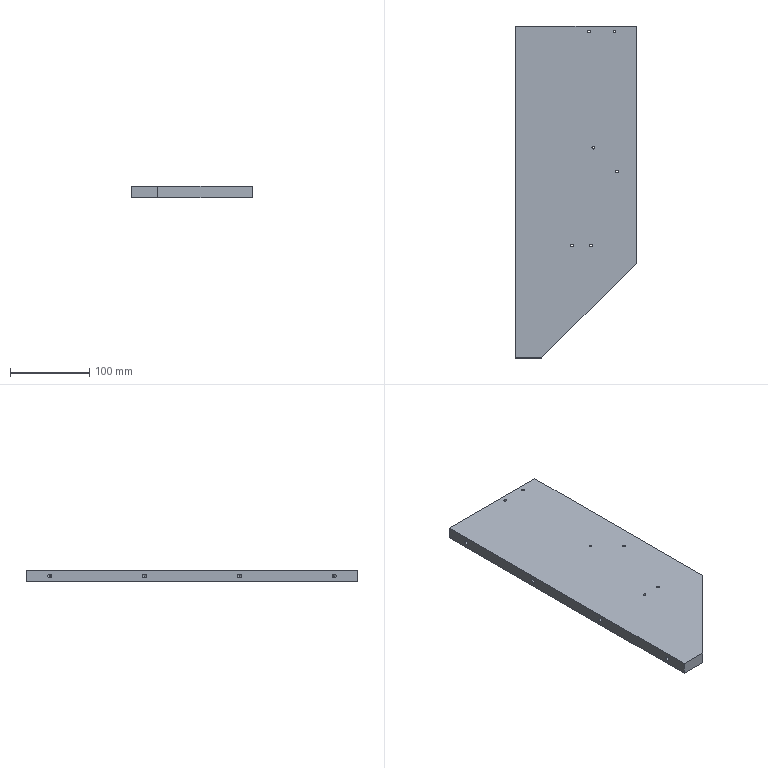Part | STEP file | KF-2212-050-006 | 1 solid | 51 faces | box 153 x 420 x 15 mm | volume 852381 mm3 | cylinder 28 | cone 16 | plane 7 | commonest cylinder face diameters 5 x16 3.3 x12
STEP:
#1=CARTESIAN_POINT('',(-3.35,-67.65,15.));
#2=VERTEX_POINT('',#1);
#3=CARTESIAN_POINT('',(-6.65,-67.65,15.));
#4=VERTEX_POINT('',#3);
#5=CARTESIAN_POINT('',(-5.,-67.65,15.));
#6=DIRECTION('',(0.,0.,-1.));
#7=DIRECTION('',(-1.,0.,0.));
#8=AXIS2_PLACEMENT_3D('',#5,#6,#7);
#9=CIRCLE('',#8,1.65);
#10=EDGE_CURVE('',#2,#4,#9,.T.);
#11=ORIENTED_EDGE('',*,*,#10,.F.);
#12=CARTESIAN_POINT('',(-3.35,-67.65,0.));
#13=VERTEX_POINT('',#12);
#14=CARTESIAN_POINT('',(-3.35,-67.65,0.));
#15=DIRECTION('',(0.,0.,-1.));
#16=VECTOR('',#15,1000.);
#17=LINE('',#14,#16);
#18=EDGE_CURVE('',#2,#13,#17,.T.);
#19=ORIENTED_EDGE('',*,*,#18,.T.);
#20=CARTESIAN_POINT('',(-6.65,-67.65,0.));
#21=VERTEX_POINT('',#20);
#22=CARTESIAN_POINT('',(-5.,-67.65,0.));
#23=DIRECTION('',(0.,0.,-1.));
#24=DIRECTION('',(-1.,0.,0.));
#25=AXIS2_PLACEMENT_3D('',#22,#23,#24);
#26=CIRCLE('',#25,1.65);
#27=EDGE_CURVE('',#13,#21,#26,.T.);
#28=ORIENTED_EDGE('',*,*,#27,.T.);
#29=CARTESIAN_POINT('',(-6.65,-67.65,0.));
#30=DIRECTION('',(0.,0.,-1.));
#31=VECTOR('',#30,1000.);
#32=LINE('',#29,#31);
#33=EDGE_CURVE('',#4,#21,#32,.T.);
#34=ORIENTED_EDGE('',*,*,#33,.F.);
#35=EDGE_LOOP('',(#11,#19,#28,#34));
#36=FACE_OUTER_BOUND('',#35,.T.);
#37=CARTESIAN_POINT('',(-5.,-67.65,0.));
#38=DIRECTION('',(0.,0.,-1.));
#39=DIRECTION('',(-1.,0.,0.));
#40=AXIS2_PLACEMENT_3D('',#37,#38,#39);
#41=CYLINDRICAL_SURFACE('',#40,1.65);
#42=ADVANCED_FACE('',(#36),#41,.F.);
#43=CARTESIAN_POINT('',(20.65,-67.65,15.));
#44=VERTEX_POINT('',#43);
#45=CARTESIAN_POINT('',(17.35,-67.65,15.));
#46=VERTEX_POINT('',#45);
#47=CARTESIAN_POINT('',(19.,-67.65,15.));
#48=DIRECTION('',(0.,0.,-1.));
#49=DIRECTION('',(-1.,0.,0.));
#50=AXIS2_PLACEMENT_3D('',#47,#48,#49);
#51=CIRCLE('',#50,1.65);
#52=EDGE_CURVE('',#44,#46,#51,.T.);
#53=ORIENTED_EDGE('',*,*,#52,.F.);
#54=CARTESIAN_POINT('',(20.65,-67.65,0.));
#55=VERTEX_POINT('',#54);
#56=CARTESIAN_POINT('',(20.65,-67.65,0.));
#57=DIRECTION('',(0.,0.,-1.));
#58=VECTOR('',#57,1000.);
#59=LINE('',#56,#58);
#60=EDGE_CURVE('',#44,#55,#59,.T.);
#61=ORIENTED_EDGE('',*,*,#60,.T.);
#62=CARTESIAN_POINT('',(17.35,-67.65,0.));
#63=VERTEX_POINT('',#62);
#64=CARTESIAN_POINT('',(19.,-67.65,0.));
#65=DIRECTION('',(0.,0.,-1.));
#66=DIRECTION('',(-1.,0.,0.));
#67=AXIS2_PLACEMENT_3D('',#64,#65,#66);
#68=CIRCLE('',#67,1.65);
#69=EDGE_CURVE('',#55,#63,#68,.T.);
#70=ORIENTED_EDGE('',*,*,#69,.T.);
#71=CARTESIAN_POINT('',(17.35,-67.65,0.));
#72=DIRECTION('',(0.,0.,-1.));
#73=VECTOR('',#72,1000.);
#74=LINE('',#71,#73);
#75=EDGE_CURVE('',#46,#63,#74,.T.);
#76=ORIENTED_EDGE('',*,*,#75,.F.);
#77=EDGE_LOOP('',(#53,#61,#70,#76));
#78=FACE_OUTER_BOUND('',#77,.T.);
#79=CARTESIAN_POINT('',(19.,-67.65,0.));
#80=DIRECTION('',(0.,0.,-1.));
#81=DIRECTION('',(-1.,0.,0.));
#82=AXIS2_PLACEMENT_3D('',#79,#80,#81);
#83=CYLINDRICAL_SURFACE('',#82,1.65);
#84=ADVANCED_FACE('',(#78),#83,.F.);
#85=CARTESIAN_POINT('',(23.523,56.,15.));
#86=VERTEX_POINT('',#85);
#87=CARTESIAN_POINT('',(20.223,56.,15.));
#88=VERTEX_POINT('',#87);
#89=CARTESIAN_POINT('',(21.873,56.,15.));
#90=DIRECTION('',(0.,0.,-1.));
#91=DIRECTION('',(-1.,0.,0.));
#92=AXIS2_PLACEMENT_3D('',#89,#90,#91);
#93=CIRCLE('',#92,1.65);
#94=EDGE_CURVE('',#86,#88,#93,.T.);
#95=ORIENTED_EDGE('',*,*,#94,.F.);
#96=CARTESIAN_POINT('',(23.523,56.,0.));
#97=VERTEX_POINT('',#96);
#98=CARTESIAN_POINT('',(23.523,56.,0.));
#99=DIRECTION('',(0.,0.,-1.));
#100=VECTOR('',#99,1000.);
#101=LINE('',#98,#100);
#102=EDGE_CURVE('',#86,#97,#101,.T.);
#103=ORIENTED_EDGE('',*,*,#102,.T.);
#104=CARTESIAN_POINT('',(20.223,56.,0.));
#105=VERTEX_POINT('',#104);
#106=CARTESIAN_POINT('',(21.873,56.,0.));
#107=DIRECTION('',(0.,0.,-1.));
#108=DIRECTION('',(-1.,0.,0.));
#109=AXIS2_PLACEMENT_3D('',#106,#107,#108);
#110=CIRCLE('',#109,1.65);
#111=EDGE_CURVE('',#97,#105,#110,.T.);
#112=ORIENTED_EDGE('',*,*,#111,.T.);
#113=CARTESIAN_POINT('',(20.223,56.,0.));
#114=DIRECTION('',(0.,0.,-1.));
#115=VECTOR('',#114,1000.);
#116=LINE('',#113,#115);
#117=EDGE_CURVE('',#88,#105,#116,.T.);
#118=ORIENTED_EDGE('',*,*,#117,.F.);
#119=EDGE_LOOP('',(#95,#103,#112,#118));
#120=FACE_OUTER_BOUND('',#119,.T.);
#121=CARTESIAN_POINT('',(21.873,56.,0.));
#122=DIRECTION('',(0.,0.,-1.));
#123=DIRECTION('',(-1.,0.,0.));
#124=AXIS2_PLACEMENT_3D('',#121,#122,#123);
#125=CYLINDRICAL_SURFACE('',#124,1.65);
#126=ADVANCED_FACE('',(#120),#125,.F.);
#127=CARTESIAN_POINT('',(53.523,26.,15.));
#128=VERTEX_POINT('',#127);
#129=CARTESIAN_POINT('',(50.223,26.,15.));
#130=VERTEX_POINT('',#129);
#131=CARTESIAN_POINT('',(51.873,26.,15.));
#132=DIRECTION('',(0.,0.,-1.));
#133=DIRECTION('',(-1.,0.,0.));
#134=AXIS2_PLACEMENT_3D('',#131,#132,#133);
#135=CIRCLE('',#134,1.65);
#136=EDGE_CURVE('',#128,#130,#135,.T.);
#137=ORIENTED_EDGE('',*,*,#136,.F.);
#138=CARTESIAN_POINT('',(53.523,26.,0.));
#139=VERTEX_POINT('',#138);
#140=CARTESIAN_POINT('',(53.523,26.,0.));
#141=DIRECTION('',(0.,0.,-1.));
#142=VECTOR('',#141,1000.);
#143=LINE('',#140,#142);
#144=EDGE_CURVE('',#128,#139,#143,.T.);
#145=ORIENTED_EDGE('',*,*,#144,.T.);
#146=CARTESIAN_POINT('',(50.223,26.,0.));
#147=VERTEX_POINT('',#146);
#148=CARTESIAN_POINT('',(51.873,26.,0.));
#149=DIRECTION('',(0.,0.,-1.));
#150=DIRECTION('',(-1.,0.,0.));
#151=AXIS2_PLACEMENT_3D('',#148,#149,#150);
#152=CIRCLE('',#151,1.65);
#153=EDGE_CURVE('',#139,#147,#152,.T.);
#154=ORIENTED_EDGE('',*,*,#153,.T.);
#155=CARTESIAN_POINT('',(50.223,26.,0.));
#156=DIRECTION('',(0.,0.,-1.));
#157=VECTOR('',#156,1000.);
#158=LINE('',#155,#157);
#159=EDGE_CURVE('',#130,#147,#158,.T.);
#160=ORIENTED_EDGE('',*,*,#159,.F.);
#161=EDGE_LOOP('',(#137,#145,#154,#160));
#162=FACE_OUTER_BOUND('',#161,.T.);
#163=CARTESIAN_POINT('',(51.873,26.,0.));
#164=DIRECTION('',(0.,0.,-1.));
#165=DIRECTION('',(-1.,0.,0.));
#166=AXIS2_PLACEMENT_3D('',#163,#164,#165);
#167=CYLINDRICAL_SURFACE('',#166,1.65);
#168=ADVANCED_FACE('',(#162),#167,.F.);
#169=CARTESIAN_POINT('',(18.15,203.,15.));
#170=VERTEX_POINT('',#169);
#171=CARTESIAN_POINT('',(14.85,203.,15.));
#172=VERTEX_POINT('',#171);
#173=CARTESIAN_POINT('',(16.5,203.,15.));
#174=DIRECTION('',(0.,0.,-1.));
#175=DIRECTION('',(-1.,0.,0.));
#176=AXIS2_PLACEMENT_3D('',#173,#174,#175);
#177=CIRCLE('',#176,1.65);
#178=EDGE_CURVE('',#170,#172,#177,.T.);
#179=ORIENTED_EDGE('',*,*,#178,.F.);
#180=CARTESIAN_POINT('',(18.15,203.,0.));
#181=VERTEX_POINT('',#180);
#182=CARTESIAN_POINT('',(18.15,203.,0.));
#183=DIRECTION('',(0.,0.,-1.));
#184=VECTOR('',#183,1000.);
#185=LINE('',#182,#184);
#186=EDGE_CURVE('',#170,#181,#185,.T.);
#187=ORIENTED_EDGE('',*,*,#186,.T.);
#188=CARTESIAN_POINT('',(14.85,203.,0.));
#189=VERTEX_POINT('',#188);
#190=CARTESIAN_POINT('',(16.5,203.,0.));
#191=DIRECTION('',(0.,0.,-1.));
#192=DIRECTION('',(-1.,0.,0.));
#193=AXIS2_PLACEMENT_3D('',#190,#191,#192);
#194=CIRCLE('',#193,1.65);
#195=EDGE_CURVE('',#181,#189,#194,.T.);
#196=ORIENTED_EDGE('',*,*,#195,.T.);
#197=CARTESIAN_POINT('',(14.85,203.,0.));
#198=DIRECTION('',(0.,0.,-1.));
#199=VECTOR('',#198,1000.);
#200=LINE('',#197,#199);
#201=EDGE_CURVE('',#172,#189,#200,.T.);
#202=ORIENTED_EDGE('',*,*,#201,.F.);
#203=EDGE_LOOP('',(#179,#187,#196,#202));
#204=FACE_OUTER_BOUND('',#203,.T.);
#205=CARTESIAN_POINT('',(16.5,203.,0.));
#206=DIRECTION('',(0.,0.,-1.));
#207=DIRECTION('',(-1.,0.,0.));
#208=AXIS2_PLACEMENT_3D('',#205,#206,#207);
#209=CYLINDRICAL_SURFACE('',#208,1.65);
#210=ADVANCED_FACE('',(#204),#209,.F.);
#211=CARTESIAN_POINT('',(50.15,203.,15.));
#212=VERTEX_POINT('',#211);
#213=CARTESIAN_POINT('',(46.85,203.,15.));
#214=VERTEX_POINT('',#213);
#215=CARTESIAN_POINT('',(48.5,203.,15.));
#216=DIRECTION('',(0.,0.,-1.));
#217=DIRECTION('',(-1.,0.,0.));
#218=AXIS2_PLACEMENT_3D('',#215,#216,#217);
#219=CIRCLE('',#218,1.65);
#220=EDGE_CURVE('',#212,#214,#219,.T.);
#221=ORIENTED_EDGE('',*,*,#220,.F.);
#222=CARTESIAN_POINT('',(50.15,203.,0.));
#223=VERTEX_POINT('',#222);
#224=CARTESIAN_POINT('',(50.15,203.,0.));
#225=DIRECTION('',(0.,0.,-1.));
#226=VECTOR('',#225,1000.);
#227=LINE('',#224,#226);
#228=EDGE_CURVE('',#212,#223,#227,.T.);
#229=ORIENTED_EDGE('',*,*,#228,.T.);
#230=CARTESIAN_POINT('',(46.85,203.,0.));
#231=VERTEX_POINT('',#230);
#232=CARTESIAN_POINT('',(48.5,203.,0.));
#233=DIRECTION('',(0.,0.,-1.));
#234=DIRECTION('',(-1.,0.,0.));
#235=AXIS2_PLACEMENT_3D('',#232,#233,#234);
#236=CIRCLE('',#235,1.65);
#237=EDGE_CURVE('',#223,#231,#236,.T.);
#238=ORIENTED_EDGE('',*,*,#237,.T.);
#239=CARTESIAN_POINT('',(46.85,203.,0.));
#240=DIRECTION('',(0.,0.,-1.));
#241=VECTOR('',#240,1000.);
#242=LINE('',#239,#241);
#243=EDGE_CURVE('',#214,#231,#242,.T.);
#244=ORIENTED_EDGE('',*,*,#243,.F.);
#245=EDGE_LOOP('',(#221,#229,#238,#244));
#246=FACE_OUTER_BOUND('',#245,.T.);
#247=CARTESIAN_POINT('',(48.5,203.,0.));
#248=DIRECTION('',(0.,0.,-1.));
#249=DIRECTION('',(-1.,0.,0.));
#250=AXIS2_PLACEMENT_3D('',#247,#248,#249);
#251=CYLINDRICAL_SURFACE('',#250,1.65);
#252=ADVANCED_FACE('',(#246),#251,.F.);
#253=CARTESIAN_POINT('',(59.5,-75.,10.));
#254=VERTEX_POINT('',#253);
#255=CARTESIAN_POINT('',(59.5,-75.,5.));
#256=VERTEX_POINT('',#255);
#257=CARTESIAN_POINT('',(59.5,-75.,7.5));
#258=DIRECTION('',(1.,0.,0.));
#259=DIRECTION('',(0.,0.,-1.));
#260=AXIS2_PLACEMENT_3D('',#257,#258,#259);
#261=CIRCLE('',#260,2.5);
#262=EDGE_CURVE('',#254,#256,#261,.T.);
#263=ORIENTED_EDGE('',*,*,#262,.F.);
#264=CARTESIAN_POINT('',(76.5,-75.,10.));
#265=VERTEX_POINT('',#264);
#266=CARTESIAN_POINT('',(76.5,-75.,10.));
#267=DIRECTION('',(1.,0.,0.));
#268=VECTOR('',#267,1000.);
#269=LINE('',#266,#268);
#270=EDGE_CURVE('',#254,#265,#269,.T.);
#271=ORIENTED_EDGE('',*,*,#270,.T.);
#272=CARTESIAN_POINT('',(76.5,-75.,5.));
#273=VERTEX_POINT('',#272);
#274=CARTESIAN_POINT('',(76.5,-75.,7.5));
#275=DIRECTION('',(1.,0.,0.));
#276=DIRECTION('',(0.,0.,-1.));
#277=AXIS2_PLACEMENT_3D('',#274,#275,#276);
#278=CIRCLE('',#277,2.5);
#279=EDGE_CURVE('',#265,#273,#278,.T.);
#280=ORIENTED_EDGE('',*,*,#279,.T.);
#281=CARTESIAN_POINT('',(76.5,-75.,5.));
#282=DIRECTION('',(1.,0.,0.));
#283=VECTOR('',#282,1000.);
#284=LINE('',#281,#283);
#285=EDGE_CURVE('',#256,#273,#284,.T.);
#286=ORIENTED_EDGE('',*,*,#285,.F.);
#287=EDGE_LOOP('',(#263,#271,#280,#286));
#288=FACE_OUTER_BOUND('',#287,.T.);
#289=CARTESIAN_POINT('',(76.5,-75.,7.5));
#290=DIRECTION('',(1.,0.,0.));
#291=DIRECTION('',(0.,0.,-1.));
#292=AXIS2_PLACEMENT_3D('',#289,#290,#291);
#293=CYLINDRICAL_SURFACE('',#292,2.5);
#294=ADVANCED_FACE('',(#288),#293,.F.);
#295=CARTESIAN_POINT('',(57.998,-75.,7.5));
#296=VERTEX_POINT('',#295);
#297=CARTESIAN_POINT('',(59.5,-75.,5.));
#298=DIRECTION('',(0.515,0.,-0.8572));
#299=VECTOR('',#298,1000.);
#300=LINE('',#297,#299);
#301=EDGE_CURVE('',#296,#256,#300,.T.);
#302=ORIENTED_EDGE('',*,*,#301,.F.);
#303=CARTESIAN_POINT('',(59.5,-75.,10.));
#304=DIRECTION('',(0.515,0.,0.8572));
#305=VECTOR('',#304,1000.);
#306=LINE('',#303,#305);
#307=EDGE_CURVE('',#296,#254,#306,.T.);
#308=ORIENTED_EDGE('',*,*,#307,.T.);
#309=ORIENTED_EDGE('',*,*,#262,.T.);
#310=EDGE_LOOP('',(#302,#308,#309));
#311=FACE_OUTER_BOUND('',#310,.T.);
#312=CARTESIAN_POINT('',(59.5,-75.,7.5));
#313=DIRECTION('',(1.,0.,0.));
#314=DIRECTION('',(0.,0.,-1.));
#315=AXIS2_PLACEMENT_3D('',#312,#313,#314);
#316=CONICAL_SURFACE('',#315,2.5,1.03);
#317=ADVANCED_FACE('',(#311),#316,.F.);
#318=CARTESIAN_POINT('',(59.5,15.,10.));
#319=VERTEX_POINT('',#318);
#320=CARTESIAN_POINT('',(59.5,15.,5.));
#321=VERTEX_POINT('',#320);
#322=CARTESIAN_POINT('',(59.5,15.,7.5));
#323=DIRECTION('',(1.,0.,0.));
#324=DIRECTION('',(0.,0.,-1.));
#325=AXIS2_PLACEMENT_3D('',#322,#323,#324);
#326=CIRCLE('',#325,2.5);
#327=EDGE_CURVE('',#319,#321,#326,.T.);
#328=ORIENTED_EDGE('',*,*,#327,.F.);
#329=CARTESIAN_POINT('',(76.5,15.,10.));
#330=VERTEX_POINT('',#329);
#331=CARTESIAN_POINT('',(76.5,15.,10.));
#332=DIRECTION('',(1.,0.,0.));
#333=VECTOR('',#332,1000.);
#334=LINE('',#331,#333);
#335=EDGE_CURVE('',#319,#330,#334,.T.);
#336=ORIENTED_EDGE('',*,*,#335,.T.);
#337=CARTESIAN_POINT('',(76.5,15.,5.));
#338=VERTEX_POINT('',#337);
#339=CARTESIAN_POINT('',(76.5,15.,7.5));
#340=DIRECTION('',(1.,0.,0.));
#341=DIRECTION('',(0.,0.,-1.));
#342=AXIS2_PLACEMENT_3D('',#339,#340,#341);
#343=CIRCLE('',#342,2.5);
#344=EDGE_CURVE('',#330,#338,#343,.T.);
#345=ORIENTED_EDGE('',*,*,#344,.T.);
#346=CARTESIAN_POINT('',(76.5,15.,5.));
#347=DIRECTION('',(1.,0.,0.));
#348=VECTOR('',#347,1000.);
#349=LINE('',#346,#348);
#350=EDGE_CURVE('',#321,#338,#349,.T.);
#351=ORIENTED_EDGE('',*,*,#350,.F.);
#352=EDGE_LOOP('',(#328,#336,#345,#351));
#353=FACE_OUTER_BOUND('',#352,.T.);
#354=CARTESIAN_POINT('',(76.5,15.,7.5));
#355=DIRECTION('',(1.,0.,0.));
#356=DIRECTION('',(0.,0.,-1.));
#357=AXIS2_PLACEMENT_3D('',#354,#355,#356);
#358=CYLINDRICAL_SURFACE('',#357,2.5);
#359=ADVANCED_FACE('',(#353),#358,.F.);
#360=CARTESIAN_POINT('',(57.998,15.,7.5));
#361=VERTEX_POINT('',#360);
#362=CARTESIAN_POINT('',(59.5,15.,5.));
#363=DIRECTION('',(0.515,0.,-0.8572));
#364=VECTOR('',#363,1000.);
#365=LINE('',#362,#364);
#366=EDGE_CURVE('',#361,#321,#365,.T.);
#367=ORIENTED_EDGE('',*,*,#366,.F.);
#368=CARTESIAN_POINT('',(59.5,15.,10.));
#369=DIRECTION('',(0.515,0.,0.8572));
#370=VECTOR('',#369,1000.);
#371=LINE('',#368,#370);
#372=EDGE_CURVE('',#361,#319,#371,.T.);
#373=ORIENTED_EDGE('',*,*,#372,.T.);
#374=ORIENTED_EDGE('',*,*,#327,.T.);
#375=EDGE_LOOP('',(#367,#373,#374));
#376=FACE_OUTER_BOUND('',#375,.T.);
#377=CARTESIAN_POINT('',(59.5,15.,7.5));
#378=DIRECTION('',(1.,0.,0.));
#379=DIRECTION('',(0.,0.,-1.));
#380=AXIS2_PLACEMENT_3D('',#377,#378,#379);
#381=CONICAL_SURFACE('',#380,2.5,1.03);
#382=ADVANCED_FACE('',(#376),#381,.F.);
#383=CARTESIAN_POINT('',(59.5,105.,10.));
#384=VERTEX_POINT('',#383);
#385=CARTESIAN_POINT('',(59.5,105.,5.));
#386=VERTEX_POINT('',#385);
#387=CARTESIAN_POINT('',(59.5,105.,7.5));
#388=DIRECTION('',(1.,0.,0.));
#389=DIRECTION('',(0.,0.,-1.));
#390=AXIS2_PLACEMENT_3D('',#387,#388,#389);
#391=CIRCLE('',#390,2.5);
#392=EDGE_CURVE('',#384,#386,#391,.T.);
#393=ORIENTED_EDGE('',*,*,#392,.F.);
#394=CARTESIAN_POINT('',(76.5,105.,10.));
#395=VERTEX_POINT('',#394);
#396=CARTESIAN_POINT('',(76.5,105.,10.));
#397=DIRECTION('',(1.,0.,0.));
#398=VECTOR('',#397,1000.);
#399=LINE('',#396,#398);
#400=EDGE_CURVE('',#384,#395,#399,.T.);
#401=ORIENTED_EDGE('',*,*,#400,.T.);
#402=CARTESIAN_POINT('',(76.5,105.,5.));
#403=VERTEX_POINT('',#402);
#404=CARTESIAN_POINT('',(76.5,105.,7.5));
#405=DIRECTION('',(1.,0.,0.));
#406=DIRECTION('',(0.,0.,-1.));
#407=AXIS2_PLACEMENT_3D('',#404,#405,#406);
#408=CIRCLE('',#407,2.5);
#409=EDGE_CURVE('',#395,#403,#408,.T.);
#410=ORIENTED_EDGE('',*,*,#409,.T.);
#411=CARTESIAN_POINT('',(76.5,105.,5.));
#412=DIRECTION('',(1.,0.,0.));
#413=VECTOR('',#412,1000.);
#414=LINE('',#411,#413);
#415=EDGE_CURVE('',#386,#403,#414,.T.);
#416=ORIENTED_EDGE('',*,*,#415,.F.);
#417=EDGE_LOOP('',(#393,#401,#410,#416));
#418=FACE_OUTER_BOUND('',#417,.T.);
#419=CARTESIAN_POINT('',(76.5,105.,7.5));
#420=DIRECTION('',(1.,0.,0.));
#421=DIRECTION('',(0.,0.,-1.));
#422=AXIS2_PLACEMENT_3D('',#419,#420,#421);
#423=CYLINDRICAL_SURFACE('',#422,2.5);
#424=ADVANCED_FACE('',(#418),#423,.F.);
#425=CARTESIAN_POINT('',(57.998,105.,7.5));
#426=VERTEX_POINT('',#425);
#427=CARTESIAN_POINT('',(59.5,105.,5.));
#428=DIRECTION('',(0.515,0.,-0.8572));
#429=VECTOR('',#428,1000.);
#430=LINE('',#427,#429);
#431=EDGE_CURVE('',#426,#386,#430,.T.);
#432=ORIENTED_EDGE('',*,*,#431,.F.);
#433=CARTESIAN_POINT('',(59.5,105.,10.));
#434=DIRECTION('',(0.515,0.,0.8572));
#435=VECTOR('',#434,1000.);
#436=LINE('',#433,#435);
#437=EDGE_CURVE('',#426,#384,#436,.T.);
#438=ORIENTED_EDGE('',*,*,#437,.T.);
#439=ORIENTED_EDGE('',*,*,#392,.T.);
#440=EDGE_LOOP('',(#432,#438,#439));
#441=FACE_OUTER_BOUND('',#440,.T.);
#442=CARTESIAN_POINT('',(59.5,105.,7.5));
#443=DIRECTION('',(1.,0.,0.));
#444=DIRECTION('',(0.,0.,-1.));
#445=AXIS2_PLACEMENT_3D('',#442,#443,#444);
#446=CONICAL_SURFACE('',#445,2.5,1.03);
#447=ADVANCED_FACE('',(#441),#446,.F.);
#448=CARTESIAN_POINT('',(59.5,195.,10.));
#449=VERTEX_POINT('',#448);
#450=CARTESIAN_POINT('',(59.5,195.,5.));
#451=VERTEX_POINT('',#450);
#452=CARTESIAN_POINT('',(59.5,195.,7.5));
#453=DIRECTION('',(1.,0.,0.));
#454=DIRECTION('',(0.,0.,-1.));
#455=AXIS2_PLACEMENT_3D('',#452,#453,#454);
#456=CIRCLE('',#455,2.5);
#457=EDGE_CURVE('',#449,#451,#456,.T.);
#458=ORIENTED_EDGE('',*,*,#457,.F.);
#459=CARTESIAN_POINT('',(76.5,195.,10.));
#460=VERTEX_POINT('',#459);
#461=CARTESIAN_POINT('',(76.5,195.,10.));
#462=DIRECTION('',(1.,0.,0.));
#463=VECTOR('',#462,1000.);
#464=LINE('',#461,#463);
#465=EDGE_CURVE('',#449,#460,#464,.T.);
#466=ORIENTED_EDGE('',*,*,#465,.T.);
#467=CARTESIAN_POINT('',(76.5,195.,5.));
#468=VERTEX_POINT('',#467);
#469=CARTESIAN_POINT('',(76.5,195.,7.5));
#470=DIRECTION('',(1.,0.,0.));
#471=DIRECTION('',(0.,0.,-1.));
#472=AXIS2_PLACEMENT_3D('',#469,#470,#471);
#473=CIRCLE('',#472,2.5);
#474=EDGE_CURVE('',#460,#468,#473,.T.);
#475=ORIENTED_EDGE('',*,*,#474,.T.);
#476=CARTESIAN_POINT('',(76.5,195.,5.));
#477=DIRECTION('',(1.,0.,0.));
#478=VECTOR('',#477,1000.);
#479=LINE('',#476,#478);
#480=EDGE_CURVE('',#451,#468,#479,.T.);
#481=ORIENTED_EDGE('',*,*,#480,.F.);
#482=EDGE_LOOP('',(#458,#466,#475,#481));
#483=FACE_OUTER_BOUND('',#482,.T.);
#484=CARTESIAN_POINT('',(76.5,195.,7.5));
#485=DIRECTION('',(1.,0.,0.));
#486=DIRECTION('',(0.,0.,-1.));
#487=AXIS2_PLACEMENT_3D('',#484,#485,#486);
#488=CYLINDRICAL_SURFACE('',#487,2.5);
#489=ADVANCED_FACE('',(#483),#488,.F.);
#490=CARTESIAN_POINT('',(57.998,195.,7.5));
#491=VERTEX_POINT('',#490);
#492=CARTESIAN_POINT('',(59.5,195.,5.));
#493=DIRECTION('',(0.515,0.,-0.8572));
#494=VECTOR('',#493,1000.);
#495=LINE('',#492,#494);
#496=EDGE_CURVE('',#491,#451,#495,.T.);
#497=ORIENTED_EDGE('',*,*,#496,.F.);
#498=CARTESIAN_POINT('',(59.5,195.,10.));
#499=DIRECTION('',(0.515,0.,0.8572));
#500=VECTOR('',#499,1000.);
#501=LINE('',#498,#500);
#502=EDGE_CURVE('',#491,#449,#501,.T.);
#503=ORIENTED_EDGE('',*,*,#502,.T.);
#504=ORIENTED_EDGE('',*,*,#457,.T.);
#505=EDGE_LOOP('',(#497,#503,#504));
#506=FACE_OUTER_BOUND('',#505,.T.);
#507=CARTESIAN_POINT('',(59.5,195.,7.5));
#508=DIRECTION('',(1.,0.,0.));
#509=DIRECTION('',(0.,0.,-1.));
#510=AXIS2_PLACEMENT_3D('',#507,#508,#509);
#511=CONICAL_SURFACE('',#510,2.5,1.03);
#512=ADVANCED_FACE('',(#506),#511,.F.);
#513=CARTESIAN_POINT('',(-59.5,180.,5.));
#514=VERTEX_POINT('',#513);
#515=CARTESIAN_POINT('',(-59.5,180.,10.));
#516=VERTEX_POINT('',#515);
#517=CARTESIAN_POINT('',(-59.5,180.,7.5));
#518=DIRECTION('',(-1.,0.,0.));
#519=DIRECTION('',(0.,0.,1.));
#520=AXIS2_PLACEMENT_3D('',#517,#518,#519);
#521=CIRCLE('',#520,2.5);
#522=EDGE_CURVE('',#514,#516,#521,.T.);
#523=ORIENTED_EDGE('',*,*,#522,.F.);
#524=CARTESIAN_POINT('',(-76.5,180.,5.));
#525=VERTEX_POINT('',#524);
#526=CARTESIAN_POINT('',(-76.5,180.,5.));
#527=DIRECTION('',(-1.,0.,0.));
#528=VECTOR('',#527,1000.);
#529=LINE('',#526,#528);
#530=EDGE_CURVE('',#514,#525,#529,.T.);
#531=ORIENTED_EDGE('',*,*,#530,.T.);
#532=CARTESIAN_POINT('',(-76.5,180.,10.));
#533=VERTEX_POINT('',#532);
#534=CARTESIAN_POINT('',(-76.5,180.,7.5));
#535=DIRECTION('',(-1.,0.,0.));
#536=DIRECTION('',(0.,0.,1.));
#537=AXIS2_PLACEMENT_3D('',#534,#535,#536);
#538=CIRCLE('',#537,2.5);
#539=EDGE_CURVE('',#525,#533,#538,.T.);
#540=ORIENTED_EDGE('',*,*,#539,.T.);
#541=CARTESIAN_POINT('',(-76.5,180.,10.));
#542=DIRECTION('',(-1.,0.,0.));
#543=VECTOR('',#542,1000.);
#544=LINE('',#541,#543);
#545=EDGE_CURVE('',#516,#533,#544,.T.);
#546=ORIENTED_EDGE('',*,*,#545,.F.);
#547=EDGE_LOOP('',(#523,#531,#540,#546));
#548=FACE_OUTER_BOUND('',#547,.T.);
#549=CARTESIAN_POINT('',(-76.5,180.,7.5));
#550=DIRECTION('',(-1.,0.,0.));
#551=DIRECTION('',(0.,0.,1.));
#552=AXIS2_PLACEMENT_3D('',#549,#550,#551);
#553=CYLINDRICAL_SURFACE('',#552,2.5);
#554=ADVANCED_FACE('',(#548),#553,.F.);
#555=CARTESIAN_POINT('',(-57.998,180.,7.5));
#556=VERTEX_POINT('',#555);
#557=CARTESIAN_POINT('',(-59.5,180.,10.));
#558=DIRECTION('',(-0.515,0.,0.8572));
#559=VECTOR('',#558,1000.);
#560=LINE('',#557,#559);
#561=EDGE_CURVE('',#556,#516,#560,.T.);
#562=ORIENTED_EDGE('',*,*,#561,.F.);
#563=CARTESIAN_POINT('',(-59.5,180.,5.));
#564=DIRECTION('',(-0.515,0.,-0.8572));
#565=VECTOR('',#564,1000.);
#566=LINE('',#563,#565);
#567=EDGE_CURVE('',#556,#514,#566,.T.);
#568=ORIENTED_EDGE('',*,*,#567,.T.);
#569=ORIENTED_EDGE('',*,*,#522,.T.);
#570=EDGE_LOOP('',(#562,#568,#569));
#571=FACE_OUTER_BOUND('',#570,.T.);
#572=CARTESIAN_POINT('',(-59.5,180.,7.5));
#573=DIRECTION('',(-1.,0.,0.));
#574=DIRECTION('',(0.,0.,1.));
#575=AXIS2_PLACEMENT_3D('',#572,#573,#574);
#576=CONICAL_SURFACE('',#575,2.5,1.03);
#577=ADVANCED_FACE('',(#571),#576,.F.);
#578=CARTESIAN_POINT('',(-59.5,60.,5.));
#579=VERTEX_POINT('',#578);
#580=CARTESIAN_POINT('',(-59.5,60.,10.));
#581=VERTEX_POINT('',#580);
#582=CARTESIAN_POINT('',(-59.5,60.,7.5));
#583=DIRECTION('',(-1.,0.,0.));
#584=DIRECTION('',(0.,0.,1.));
#585=AXIS2_PLACEMENT_3D('',#582,#583,#584);
#586=CIRCLE('',#585,2.5);
#587=EDGE_CURVE('',#579,#581,#586,.T.);
#588=ORIENTED_EDGE('',*,*,#587,.F.);
#589=CARTESIAN_POINT('',(-76.5,60.,5.));
#590=VERTEX_POINT('',#589);
#591=CARTESIAN_POINT('',(-76.5,60.,5.));
#592=DIRECTION('',(-1.,0.,0.));
#593=VECTOR('',#592,1000.);
#594=LINE('',#591,#593);
#595=EDGE_CURVE('',#579,#590,#594,.T.);
#596=ORIENTED_EDGE('',*,*,#595,.T.);
#597=CARTESIAN_POINT('',(-76.5,60.,10.));
#598=VERTEX_POINT('',#597);
#599=CARTESIAN_POINT('',(-76.5,60.,7.5));
#600=DIRECTION('',(-1.,0.,0.));
#601=DIRECTION('',(0.,0.,1.));
#602=AXIS2_PLACEMENT_3D('',#599,#600,#601);
#603=CIRCLE('',#602,2.5);
#604=EDGE_CURVE('',#590,#598,#603,.T.);
#605=ORIENTED_EDGE('',*,*,#604,.T.);
#606=CARTESIAN_POINT('',(-76.5,60.,10.));
#607=DIRECTION('',(-1.,0.,0.));
#608=VECTOR('',#607,1000.);
#609=LINE('',#606,#608);
#610=EDGE_CURVE('',#581,#598,#609,.T.);
#611=ORIENTED_EDGE('',*,*,#610,.F.);
#612=EDGE_LOOP('',(#588,#596,#605,#611));
#613=FACE_OUTER_BOUND('',#612,.T.);
#614=CARTESIAN_POINT('',(-76.5,60.,7.5));
#615=DIRECTION('',(-1.,0.,0.));
#616=DIRECTION('',(0.,0.,1.));
#617=AXIS2_PLACEMENT_3D('',#614,#615,#616);
#618=CYLINDRICAL_SURFACE('',#617,2.5);
#619=ADVANCED_FACE('',(#613),#618,.F.);
#620=CARTESIAN_POINT('',(-57.998,60.,7.5));
#621=VERTEX_POINT('',#620);
#622=CARTESIAN_POINT('',(-59.5,60.,10.));
#623=DIRECTION('',(-0.515,0.,0.8572));
#624=VECTOR('',#623,1000.);
#625=LINE('',#622,#624);
#626=EDGE_CURVE('',#621,#581,#625,.T.);
#627=ORIENTED_EDGE('',*,*,#626,.F.);
#628=CARTESIAN_POINT('',(-59.5,60.,5.));
#629=DIRECTION('',(-0.515,0.,-0.8572));
#630=VECTOR('',#629,1000.);
#631=LINE('',#628,#630);
#632=EDGE_CURVE('',#621,#579,#631,.T.);
#633=ORIENTED_EDGE('',*,*,#632,.T.);
#634=ORIENTED_EDGE('',*,*,#587,.T.);
#635=EDGE_LOOP('',(#627,#633,#634));
#636=FACE_OUTER_BOUND('',#635,.T.);
#637=CARTESIAN_POINT('',(-59.5,60.,7.5));
#638=DIRECTION('',(-1.,0.,0.));
#639=DIRECTION('',(0.,0.,1.));
#640=AXIS2_PLACEMENT_3D('',#637,#638,#639);
#641=CONICAL_SURFACE('',#640,2.5,1.03);
#642=ADVANCED_FACE('',(#636),#641,.F.);
#643=CARTESIAN_POINT('',(-59.5,-60.,5.));
#644=VERTEX_POINT('',#643);
#645=CARTESIAN_POINT('',(-59.5,-60.,10.));
#646=VERTEX_POINT('',#645);
#647=CARTESIAN_POINT('',(-59.5,-60.,7.5));
#648=DIRECTION('',(-1.,0.,0.));
#649=DIRECTION('',(0.,0.,1.));
#650=AXIS2_PLACEMENT_3D('',#647,#648,#649);
#651=CIRCLE('',#650,2.5);
#652=EDGE_CURVE('',#644,#646,#651,.T.);
#653=ORIENTED_EDGE('',*,*,#652,.F.);
#654=CARTESIAN_POINT('',(-76.5,-60.,5.));
#655=VERTEX_POINT('',#654);
#656=CARTESIAN_POINT('',(-76.5,-60.,5.));
#657=DIRECTION('',(-1.,0.,0.));
#658=VECTOR('',#657,1000.);
#659=LINE('',#656,#658);
#660=EDGE_CURVE('',#644,#655,#659,.T.);
#661=ORIENTED_EDGE('',*,*,#660,.T.);
#662=CARTESIAN_POINT('',(-76.5,-60.,10.));
#663=VERTEX_POINT('',#662);
#664=CARTESIAN_POINT('',(-76.5,-60.,7.5));
#665=DIRECTION('',(-1.,0.,0.));
#666=DIRECTION('',(0.,0.,1.));
#667=AXIS2_PLACEMENT_3D('',#664,#665,#666);
#668=CIRCLE('',#667,2.5);
#669=EDGE_CURVE('',#655,#663,#668,.T.);
#670=ORIENTED_EDGE('',*,*,#669,.T.);
#671=CARTESIAN_POINT('',(-76.5,-60.,10.));
#672=DIRECTION('',(-1.,0.,0.));
#673=VECTOR('',#672,1000.);
#674=LINE('',#671,#673);
#675=EDGE_CURVE('',#646,#663,#674,.T.);
#676=ORIENTED_EDGE('',*,*,#675,.F.);
#677=EDGE_LOOP('',(#653,#661,#670,#676));
#678=FACE_OUTER_BOUND('',#677,.T.);
#679=CARTESIAN_POINT('',(-76.5,-60.,7.5));
#680=DIRECTION('',(-1.,0.,0.));
#681=DIRECTION('',(0.,0.,1.));
#682=AXIS2_PLACEMENT_3D('',#679,#680,#681);
#683=CYLINDRICAL_SURFACE('',#682,2.5);
#684=ADVANCED_FACE('',(#678),#683,.F.);
#685=CARTESIAN_POINT('',(-57.998,-60.,7.5));
#686=VERTEX_POINT('',#685);
#687=CARTESIAN_POINT('',(-59.5,-60.,10.));
#688=DIRECTION('',(-0.515,0.,0.8572));
#689=VECTOR('',#688,1000.);
#690=LINE('',#687,#689);
#691=EDGE_CURVE('',#686,#646,#690,.T.);
#692=ORIENTED_EDGE('',*,*,#691,.F.);
#693=CARTESIAN_POINT('',(-59.5,-60.,5.));
#694=DIRECTION('',(-0.515,0.,-0.8572));
#695=VECTOR('',#694,1000.);
#696=LINE('',#693,#695);
#697=EDGE_CURVE('',#686,#644,#696,.T.);
#698=ORIENTED_EDGE('',*,*,#697,.T.);
#699=ORIENTED_EDGE('',*,*,#652,.T.);
#700=EDGE_LOOP('',(#692,#698,#699));
#701=FACE_OUTER_BOUND('',#700,.T.);
#702=CARTESIAN_POINT('',(-59.5,-60.,7.5));
#703=DIRECTION('',(-1.,0.,0.));
#704=DIRECTION('',(0.,0.,1.));
#705=AXIS2_PLACEMENT_3D('',#702,#703,#704);
#706=CONICAL_SURFACE('',#705,2.5,1.03);
#707=ADVANCED_FACE('',(#701),#706,.F.);
#708=CARTESIAN_POINT('',(-59.5,-180.,5.));
#709=VERTEX_POINT('',#708);
#710=CARTESIAN_POINT('',(-59.5,-180.,10.));
#711=VERTEX_POINT('',#710);
#712=CARTESIAN_POINT('',(-59.5,-180.,7.5));
#713=DIRECTION('',(-1.,0.,0.));
#714=DIRECTION('',(0.,0.,1.));
#715=AXIS2_PLACEMENT_3D('',#712,#713,#714);
#716=CIRCLE('',#715,2.5);
#717=EDGE_CURVE('',#709,#711,#716,.T.);
#718=ORIENTED_EDGE('',*,*,#717,.F.);
#719=CARTESIAN_POINT('',(-76.5,-180.,5.));
#720=VERTEX_POINT('',#719);
#721=CARTESIAN_POINT('',(-76.5,-180.,5.));
#722=DIRECTION('',(-1.,0.,0.));
#723=VECTOR('',#722,1000.);
#724=LINE('',#721,#723);
#725=EDGE_CURVE('',#709,#720,#724,.T.);
#726=ORIENTED_EDGE('',*,*,#725,.T.);
#727=CARTESIAN_POINT('',(-76.5,-180.,10.));
#728=VERTEX_POINT('',#727);
#729=CARTESIAN_POINT('',(-76.5,-180.,7.5));
#730=DIRECTION('',(-1.,0.,0.));
#731=DIRECTION('',(0.,0.,1.));
#732=AXIS2_PLACEMENT_3D('',#729,#730,#731);
#733=CIRCLE('',#732,2.5);
#734=EDGE_CURVE('',#720,#728,#733,.T.);
#735=ORIENTED_EDGE('',*,*,#734,.T.);
#736=CARTESIAN_POINT('',(-76.5,-180.,10.));
#737=DIRECTION('',(-1.,0.,0.));
#738=VECTOR('',#737,1000.);
#739=LINE('',#736,#738);
#740=EDGE_CURVE('',#711,#728,#739,.T.);
#741=ORIENTED_EDGE('',*,*,#740,.F.);
#742=EDGE_LOOP('',(#718,#726,#735,#741));
#743=FACE_OUTER_BOUND('',#742,.T.);
#744=CARTESIAN_POINT('',(-76.5,-180.,7.5));
#745=DIRECTION('',(-1.,0.,0.));
#746=DIRECTION('',(0.,0.,1.));
#747=AXIS2_PLACEMENT_3D('',#744,#745,#746);
#748=CYLINDRICAL_SURFACE('',#747,2.5);
#749=ADVANCED_FACE('',(#743),#748,.F.);
#750=CARTESIAN_POINT('',(-57.998,-180.,7.5));
#751=VERTEX_POINT('',#750);
#752=CARTESIAN_POINT('',(-59.5,-180.,10.));
#753=DIRECTION('',(-0.515,0.,0.8572));
#754=VECTOR('',#753,1000.);
#755=LINE('',#752,#754);
#756=EDGE_CURVE('',#751,#711,#755,.T.);
#757=ORIENTED_EDGE('',*,*,#756,.F.);
#758=CARTESIAN_POINT('',(-59.5,-180.,5.));
#759=DIRECTION('',(-0.515,0.,-0.8572));
#760=VECTOR('',#759,1000.);
#761=LINE('',#758,#760);
#762=EDGE_CURVE('',#751,#709,#761,.T.);
#763=ORIENTED_EDGE('',*,*,#762,.T.);
#764=ORIENTED_EDGE('',*,*,#717,.T.);
#765=EDGE_LOOP('',(#757,#763,#764));
#766=FACE_OUTER_BOUND('',#765,.T.);
#767=CARTESIAN_POINT('',(-59.5,-180.,7.5));
#768=DIRECTION('',(-1.,0.,0.));
#769=DIRECTION('',(0.,0.,1.));
#770=AXIS2_PLACEMENT_3D('',#767,#768,#769);
#771=CONICAL_SURFACE('',#770,2.5,1.03);
#772=ADVANCED_FACE('',(#766),#771,.F.);
#773=CARTESIAN_POINT('',(-76.5,180.,7.5));
#774=DIRECTION('',(-1.,0.,0.));
#775=DIRECTION('',(0.,0.,1.));
#776=AXIS2_PLACEMENT_3D('',#773,#774,#775);
#777=CIRCLE('',#776,2.5);
#778=EDGE_CURVE('',#533,#525,#777,.T.);
#779=ORIENTED_EDGE('',*,*,#778,.F.);
#780=ORIENTED_EDGE('',*,*,#539,.F.);
#781=EDGE_LOOP('',(#779,#780));
#782=FACE_BOUND('',#781,.T.);
#783=CARTESIAN_POINT('',(-76.5,60.,7.5));
#784=DIRECTION('',(-1.,0.,0.));
#785=DIRECTION('',(0.,0.,1.));
#786=AXIS2_PLACEMENT_3D('',#783,#784,#785);
#787=CIRCLE('',#786,2.5);
#788=EDGE_CURVE('',#598,#590,#787,.T.);
#789=ORIENTED_EDGE('',*,*,#788,.F.);
#790=ORIENTED_EDGE('',*,*,#604,.F.);
#791=EDGE_LOOP('',(#789,#790));
#792=FACE_BOUND('',#791,.T.);
#793=CARTESIAN_POINT('',(-76.5,-60.,7.5));
#794=DIRECTION('',(-1.,0.,0.));
#795=DIRECTION('',(0.,0.,1.));
#796=AXIS2_PLACEMENT_3D('',#793,#794,#795);
#797=CIRCLE('',#796,2.5);
#798=EDGE_CURVE('',#663,#655,#797,.T.);
#799=ORIENTED_EDGE('',*,*,#798,.F.);
#800=ORIENTED_EDGE('',*,*,#669,.F.);
#801=EDGE_LOOP('',(#799,#800));
#802=FACE_BOUND('',#801,.T.);
#803=CARTESIAN_POINT('',(-76.5,-180.,7.5));
#804=DIRECTION('',(-1.,0.,0.));
#805=DIRECTION('',(0.,0.,1.));
#806=AXIS2_PLACEMENT_3D('',#803,#804,#805);
#807=CIRCLE('',#806,2.5);
#808=EDGE_CURVE('',#728,#720,#807,.T.);
#809=ORIENTED_EDGE('',*,*,#808,.F.);
#810=ORIENTED_EDGE('',*,*,#734,.F.);
#811=EDGE_LOOP('',(#809,#810));
#812=FACE_BOUND('',#811,.T.);
#813=CARTESIAN_POINT('',(-76.5,210.,0.));
#814=VERTEX_POINT('',#813);
#815=CARTESIAN_POINT('',(-76.5,-210.,0.));
#816=VERTEX_POINT('',#815);
#817=CARTESIAN_POINT('',(-76.5,210.,0.));
#818=DIRECTION('',(0.,-1.,0.));
#819=VECTOR('',#818,1000.);
#820=LINE('',#817,#819);
#821=EDGE_CURVE('',#814,#816,#820,.T.);
#822=ORIENTED_EDGE('',*,*,#821,.T.);
#823=CARTESIAN_POINT('',(-76.5,-210.,15.));
#824=VERTEX_POINT('',#823);
#825=CARTESIAN_POINT('',(-76.5,-210.,15.));
#826=DIRECTION('',(0.,0.,-1.));
#827=VECTOR('',#826,1000.);
#828=LINE('',#825,#827);
#829=EDGE_CURVE('',#824,#816,#828,.T.);
#830=ORIENTED_EDGE('',*,*,#829,.F.);
#831=CARTESIAN_POINT('',(-76.5,210.,15.));
#832=VERTEX_POINT('',#831);
#833=CARTESIAN_POINT('',(-76.5,210.,15.));
#834=DIRECTION('',(0.,-1.,0.));
#835=VECTOR('',#834,1000.);
#836=LINE('',#833,#835);
#837=EDGE_CURVE('',#832,#824,#836,.T.);
#838=ORIENTED_EDGE('',*,*,#837,.F.);
#839=CARTESIAN_POINT('',(-76.5,210.,15.));
#840=DIRECTION('',(0.,0.,-1.));
#841=VECTOR('',#840,1000.);
#842=LINE('',#839,#841);
#843=EDGE_CURVE('',#832,#814,#842,.T.);
#844=ORIENTED_EDGE('',*,*,#843,.T.);
#845=EDGE_LOOP('',(#822,#830,#838,#844));
#846=FACE_OUTER_BOUND('',#845,.T.);
#847=CARTESIAN_POINT('',(-76.5,210.,15.));
#848=DIRECTION('',(1.,0.,0.));
#849=DIRECTION('',(0.,1.,0.));
#850=AXIS2_PLACEMENT_3D('',#847,#848,#849);
#851=PLANE('',#850);
#852=ADVANCED_FACE('',(#782,#792,#802,#812,#846),#851,.F.);
#853=CARTESIAN_POINT('',(-43.5,-210.,0.));
#854=VERTEX_POINT('',#853);
#855=CARTESIAN_POINT('',(76.5,-210.,0.));
#856=DIRECTION('',(1.,0.,0.));
#857=VECTOR('',#856,1000.);
#858=LINE('',#855,#857);
#859=EDGE_CURVE('',#816,#854,#858,.T.);
#860=ORIENTED_EDGE('',*,*,#859,.T.);
#861=CARTESIAN_POINT('',(-43.5,-210.,15.));
#862=VERTEX_POINT('',#861);
#863=CARTESIAN_POINT('',(-43.5,-210.,15.));
#864=DIRECTION('',(0.,0.,1.));
#865=VECTOR('',#864,1000.);
#866=LINE('',#863,#865);
#867=EDGE_CURVE('',#854,#862,#866,.T.);
#868=ORIENTED_EDGE('',*,*,#867,.T.);
#869=CARTESIAN_POINT('',(76.5,-210.,15.));
#870=DIRECTION('',(1.,0.,0.));
#871=VECTOR('',#870,1000.);
#872=LINE('',#869,#871);
#873=EDGE_CURVE('',#824,#862,#872,.T.);
#874=ORIENTED_EDGE('',*,*,#873,.F.);
#875=ORIENTED_EDGE('',*,*,#829,.T.);
#876=EDGE_LOOP('',(#860,#868,#874,#875));
#877=FACE_OUTER_BOUND('',#876,.T.);
#878=CARTESIAN_POINT('',(76.5,-210.,15.));
#879=DIRECTION('',(0.,1.,0.));
#880=DIRECTION('',(0.,0.,1.));
#881=AXIS2_PLACEMENT_3D('',#878,#879,#880);
#882=PLANE('',#881);
#883=ADVANCED_FACE('',(#877),#882,.F.);
#884=CARTESIAN_POINT('',(76.5,-75.,7.5));
#885=DIRECTION('',(1.,0.,0.));
#886=DIRECTION('',(0.,0.,-1.));
#887=AXIS2_PLACEMENT_3D('',#884,#885,#886);
#888=CIRCLE('',#887,2.5);
#889=EDGE_CURVE('',#273,#265,#888,.T.);
#890=ORIENTED_EDGE('',*,*,#889,.F.);
#891=ORIENTED_EDGE('',*,*,#279,.F.);
#892=EDGE_LOOP('',(#890,#891));
#893=FACE_BOUND('',#892,.T.);
#894=CARTESIAN_POINT('',(76.5,15.,7.5));
#895=DIRECTION('',(1.,0.,0.));
#896=DIRECTION('',(0.,0.,-1.));
#897=AXIS2_PLACEMENT_3D('',#894,#895,#896);
#898=CIRCLE('',#897,2.5);
#899=EDGE_CURVE('',#338,#330,#898,.T.);
#900=ORIENTED_EDGE('',*,*,#899,.F.);
#901=ORIENTED_EDGE('',*,*,#344,.F.);
#902=EDGE_LOOP('',(#900,#901));
#903=FACE_BOUND('',#902,.T.);
#904=CARTESIAN_POINT('',(76.5,105.,7.5));
#905=DIRECTION('',(1.,0.,0.));
#906=DIRECTION('',(0.,0.,-1.));
#907=AXIS2_PLACEMENT_3D('',#904,#905,#906);
#908=CIRCLE('',#907,2.5);
#909=EDGE_CURVE('',#403,#395,#908,.T.);
#910=ORIENTED_EDGE('',*,*,#909,.F.);
#911=ORIENTED_EDGE('',*,*,#409,.F.);
#912=EDGE_LOOP('',(#910,#911));
#913=FACE_BOUND('',#912,.T.);
#914=CARTESIAN_POINT('',(76.5,195.,7.5));
#915=DIRECTION('',(1.,0.,0.));
#916=DIRECTION('',(0.,0.,-1.));
#917=AXIS2_PLACEMENT_3D('',#914,#915,#916);
#918=CIRCLE('',#917,2.5);
#919=EDGE_CURVE('',#468,#460,#918,.T.);
#920=ORIENTED_EDGE('',*,*,#919,.F.);
#921=ORIENTED_EDGE('',*,*,#474,.F.);
#922=EDGE_LOOP('',(#920,#921));
#923=FACE_BOUND('',#922,.T.);
#924=CARTESIAN_POINT('',(76.5,-90.,15.));
#925=VERTEX_POINT('',#924);
#926=CARTESIAN_POINT('',(76.5,210.,15.));
#927=VERTEX_POINT('',#926);
#928=CARTESIAN_POINT('',(76.5,210.,15.));
#929=DIRECTION('',(0.,1.,0.));
#930=VECTOR('',#929,1000.);
#931=LINE('',#928,#930);
#932=EDGE_CURVE('',#925,#927,#931,.T.);
#933=ORIENTED_EDGE('',*,*,#932,.F.);
#934=CARTESIAN_POINT('',(76.5,-90.,0.));
#935=VERTEX_POINT('',#934);
#936=CARTESIAN_POINT('',(76.5,-90.,15.));
#937=DIRECTION('',(0.,0.,-1.));
#938=VECTOR('',#937,1000.);
#939=LINE('',#936,#938);
#940=EDGE_CURVE('',#925,#935,#939,.T.);
#941=ORIENTED_EDGE('',*,*,#940,.T.);
#942=CARTESIAN_POINT('',(76.5,210.,0.));
#943=VERTEX_POINT('',#942);
#944=CARTESIAN_POINT('',(76.5,210.,0.));
#945=DIRECTION('',(0.,1.,0.));
#946=VECTOR('',#945,1000.);
#947=LINE('',#944,#946);
#948=EDGE_CURVE('',#935,#943,#947,.T.);
#949=ORIENTED_EDGE('',*,*,#948,.T.);
#950=CARTESIAN_POINT('',(76.5,210.,15.));
#951=DIRECTION('',(0.,0.,-1.));
#952=VECTOR('',#951,1000.);
#953=LINE('',#950,#952);
#954=EDGE_CURVE('',#927,#943,#953,.T.);
#955=ORIENTED_EDGE('',*,*,#954,.F.);
#956=EDGE_LOOP('',(#933,#941,#949,#955));
#957=FACE_OUTER_BOUND('',#956,.T.);
#958=CARTESIAN_POINT('',(76.5,210.,15.));
#959=DIRECTION('',(-1.,0.,0.));
#960=DIRECTION('',(0.,-1.,0.));
#961=AXIS2_PLACEMENT_3D('',#958,#959,#960);
#962=PLANE('',#961);
#963=ADVANCED_FACE('',(#893,#903,#913,#923,#957),#962,.F.);
#964=CARTESIAN_POINT('',(76.5,210.,0.));
#965=DIRECTION('',(-1.,0.,0.));
#966=VECTOR('',#965,1000.);
#967=LINE('',#964,#966);
#968=EDGE_CURVE('',#943,#814,#967,.T.);
#969=ORIENTED_EDGE('',*,*,#968,.T.);
#970=ORIENTED_EDGE('',*,*,#843,.F.);
#971=CARTESIAN_POINT('',(76.5,210.,15.));
#972=DIRECTION('',(-1.,0.,0.));
#973=VECTOR('',#972,1000.);
#974=LINE('',#971,#973);
#975=EDGE_CURVE('',#927,#832,#974,.T.);
#976=ORIENTED_EDGE('',*,*,#975,.F.);
#977=ORIENTED_EDGE('',*,*,#954,.T.);
#978=EDGE_LOOP('',(#969,#970,#976,#977));
#979=FACE_OUTER_BOUND('',#978,.T.);
#980=CARTESIAN_POINT('',(76.5,210.,15.));
#981=DIRECTION('',(0.,-1.,0.));
#982=DIRECTION('',(0.,0.,-1.));
#983=AXIS2_PLACEMENT_3D('',#980,#981,#982);
#984=PLANE('',#983);
#985=ADVANCED_FACE('',(#979),#984,.F.);
#986=CARTESIAN_POINT('',(-5.,-67.65,15.));
#987=DIRECTION('',(0.,0.,-1.));
#988=DIRECTION('',(-1.,0.,0.));
#989=AXIS2_PLACEMENT_3D('',#986,#987,#988);
#990=CIRCLE('',#989,1.65);
#991=EDGE_CURVE('',#4,#2,#990,.T.);
#992=ORIENTED_EDGE('',*,*,#991,.T.);
#993=ORIENTED_EDGE('',*,*,#10,.T.);
#994=EDGE_LOOP('',(#992,#993));
#995=FACE_BOUND('',#994,.T.);
#996=CARTESIAN_POINT('',(19.,-67.65,15.));
#997=DIRECTION('',(0.,0.,-1.));
#998=DIRECTION('',(-1.,0.,0.));
#999=AXIS2_PLACEMENT_3D('',#996,#997,#998);
#1000=CIRCLE('',#999,1.65);
#1001=EDGE_CURVE('',#46,#44,#1000,.T.);
#1002=ORIENTED_EDGE('',*,*,#1001,.T.);
#1003=ORIENTED_EDGE('',*,*,#52,.T.);
#1004=EDGE_LOOP('',(#1002,#1003));
#1005=FACE_BOUND('',#1004,.T.);
#1006=CARTESIAN_POINT('',(21.873,56.,15.));
#1007=DIRECTION('',(0.,0.,-1.));
#1008=DIRECTION('',(-1.,0.,0.));
#1009=AXIS2_PLACEMENT_3D('',#1006,#1007,#1008);
#1010=CIRCLE('',#1009,1.65);
#1011=EDGE_CURVE('',#88,#86,#1010,.T.);
#1012=ORIENTED_EDGE('',*,*,#1011,.T.);
#1013=ORIENTED_EDGE('',*,*,#94,.T.);
#1014=EDGE_LOOP('',(#1012,#1013));
#1015=FACE_BOUND('',#1014,.T.);
#1016=CARTESIAN_POINT('',(51.873,26.,15.));
#1017=DIRECTION('',(0.,0.,-1.));
#1018=DIRECTION('',(-1.,0.,0.));
#1019=AXIS2_PLACEMENT_3D('',#1016,#1017,#1018);
#1020=CIRCLE('',#1019,1.65);
#1021=EDGE_CURVE('',#130,#128,#1020,.T.);
#1022=ORIENTED_EDGE('',*,*,#1021,.T.);
#1023=ORIENTED_EDGE('',*,*,#136,.T.);
#1024=EDGE_LOOP('',(#1022,#1023));
#1025=FACE_BOUND('',#1024,.T.);
#1026=CARTESIAN_POINT('',(16.5,203.,15.));
#1027=DIRECTION('',(0.,0.,-1.));
#1028=DIRECTION('',(-1.,0.,0.));
#1029=AXIS2_PLACEMENT_3D('',#1026,#1027,#1028);
#1030=CIRCLE('',#1029,1.65);
#1031=EDGE_CURVE('',#172,#170,#1030,.T.);
#1032=ORIENTED_EDGE('',*,*,#1031,.T.);
#1033=ORIENTED_EDGE('',*,*,#178,.T.);
#1034=EDGE_LOOP('',(#1032,#1033));
#1035=FACE_BOUND('',#1034,.T.);
#1036=CARTESIAN_POINT('',(48.5,203.,15.));
#1037=DIRECTION('',(0.,0.,-1.));
#1038=DIRECTION('',(-1.,0.,0.));
#1039=AXIS2_PLACEMENT_3D('',#1036,#1037,#1038);
#1040=CIRCLE('',#1039,1.65);
#1041=EDGE_CURVE('',#214,#212,#1040,.T.);
#1042=ORIENTED_EDGE('',*,*,#1041,.T.);
#1043=ORIENTED_EDGE('',*,*,#220,.T.);
#1044=EDGE_LOOP('',(#1042,#1043));
#1045=FACE_BOUND('',#1044,.T.);
#1046=ORIENTED_EDGE('',*,*,#873,.T.);
#1047=CARTESIAN_POINT('',(76.5,-90.,15.));
#1048=DIRECTION('',(0.7071,0.7071,0.));
#1049=VECTOR('',#1048,1000.);
#1050=LINE('',#1047,#1049);
#1051=EDGE_CURVE('',#862,#925,#1050,.T.);
#1052=ORIENTED_EDGE('',*,*,#1051,.T.);
#1053=ORIENTED_EDGE('',*,*,#932,.T.);
#1054=ORIENTED_EDGE('',*,*,#975,.T.);
#1055=ORIENTED_EDGE('',*,*,#837,.T.);
#1056=EDGE_LOOP('',(#1046,#1052,#1053,#1054,#1055));
#1057=FACE_OUTER_BOUND('',#1056,.T.);
#1058=CARTESIAN_POINT('',(0.,0.,15.));
#1059=DIRECTION('',(0.,0.,-1.));
#1060=DIRECTION('',(-1.,0.,0.));
#1061=AXIS2_PLACEMENT_3D('',#1058,#1059,#1060);
#1062=PLANE('',#1061);
#1063=ADVANCED_FACE('',(#995,#1005,#1015,#1025,#1035,#1045,#1057),#1062,.F.);
#1064=CARTESIAN_POINT('',(-5.,-67.65,0.));
#1065=DIRECTION('',(0.,0.,-1.));
#1066=DIRECTION('',(-1.,0.,0.));
#1067=AXIS2_PLACEMENT_3D('',#1064,#1065,#1066);
#1068=CIRCLE('',#1067,1.65);
#1069=EDGE_CURVE('',#21,#13,#1068,.T.);
#1070=ORIENTED_EDGE('',*,*,#1069,.F.);
#1071=ORIENTED_EDGE('',*,*,#27,.F.);
#1072=EDGE_LOOP('',(#1070,#1071));
#1073=FACE_BOUND('',#1072,.T.);
#1074=CARTESIAN_POINT('',(19.,-67.65,0.));
#1075=DIRECTION('',(0.,0.,-1.));
#1076=DIRECTION('',(-1.,0.,0.));
#1077=AXIS2_PLACEMENT_3D('',#1074,#1075,#1076);
#1078=CIRCLE('',#1077,1.65);
#1079=EDGE_CURVE('',#63,#55,#1078,.T.);
#1080=ORIENTED_EDGE('',*,*,#1079,.F.);
#1081=ORIENTED_EDGE('',*,*,#69,.F.);
#1082=EDGE_LOOP('',(#1080,#1081));
#1083=FACE_BOUND('',#1082,.T.);
#1084=CARTESIAN_POINT('',(21.873,56.,0.));
#1085=DIRECTION('',(0.,0.,-1.));
#1086=DIRECTION('',(-1.,0.,0.));
#1087=AXIS2_PLACEMENT_3D('',#1084,#1085,#1086);
#1088=CIRCLE('',#1087,1.65);
#1089=EDGE_CURVE('',#105,#97,#1088,.T.);
#1090=ORIENTED_EDGE('',*,*,#1089,.F.);
#1091=ORIENTED_EDGE('',*,*,#111,.F.);
#1092=EDGE_LOOP('',(#1090,#1091));
#1093=FACE_BOUND('',#1092,.T.);
#1094=CARTESIAN_POINT('',(51.873,26.,0.));
#1095=DIRECTION('',(0.,0.,-1.));
#1096=DIRECTION('',(-1.,0.,0.));
#1097=AXIS2_PLACEMENT_3D('',#1094,#1095,#1096);
#1098=CIRCLE('',#1097,1.65);
#1099=EDGE_CURVE('',#147,#139,#1098,.T.);
#1100=ORIENTED_EDGE('',*,*,#1099,.F.);
#1101=ORIENTED_EDGE('',*,*,#153,.F.);
#1102=EDGE_LOOP('',(#1100,#1101));
#1103=FACE_BOUND('',#1102,.T.);
#1104=CARTESIAN_POINT('',(16.5,203.,0.));
#1105=DIRECTION('',(0.,0.,-1.));
#1106=DIRECTION('',(-1.,0.,0.));
#1107=AXIS2_PLACEMENT_3D('',#1104,#1105,#1106);
#1108=CIRCLE('',#1107,1.65);
#1109=EDGE_CURVE('',#189,#181,#1108,.T.);
#1110=ORIENTED_EDGE('',*,*,#1109,.F.);
#1111=ORIENTED_EDGE('',*,*,#195,.F.);
#1112=EDGE_LOOP('',(#1110,#1111));
#1113=FACE_BOUND('',#1112,.T.);
#1114=CARTESIAN_POINT('',(48.5,203.,0.));
#1115=DIRECTION('',(0.,0.,-1.));
#1116=DIRECTION('',(-1.,0.,0.));
#1117=AXIS2_PLACEMENT_3D('',#1114,#1115,#1116);
#1118=CIRCLE('',#1117,1.65);
#1119=EDGE_CURVE('',#231,#223,#1118,.T.);
#1120=ORIENTED_EDGE('',*,*,#1119,.F.);
#1121=ORIENTED_EDGE('',*,*,#237,.F.);
#1122=EDGE_LOOP('',(#1120,#1121));
#1123=FACE_BOUND('',#1122,.T.);
#1124=ORIENTED_EDGE('',*,*,#948,.F.);
#1125=CARTESIAN_POINT('',(83.25,-83.25,0.));
#1126=DIRECTION('',(-0.7071,-0.7071,0.));
#1127=VECTOR('',#1126,1000.);
#1128=LINE('',#1125,#1127);
#1129=EDGE_CURVE('',#935,#854,#1128,.T.);
#1130=ORIENTED_EDGE('',*,*,#1129,.T.);
#1131=ORIENTED_EDGE('',*,*,#859,.F.);
#1132=ORIENTED_EDGE('',*,*,#821,.F.);
#1133=ORIENTED_EDGE('',*,*,#968,.F.);
#1134=EDGE_LOOP('',(#1124,#1130,#1131,#1132,#1133));
#1135=FACE_OUTER_BOUND('',#1134,.T.);
#1136=CARTESIAN_POINT('',(0.,0.,0.));
#1137=DIRECTION('',(0.,0.,-1.));
#1138=DIRECTION('',(-1.,0.,0.));
#1139=AXIS2_PLACEMENT_3D('',#1136,#1137,#1138);
#1140=PLANE('',#1139);
#1141=ADVANCED_FACE('',(#1073,#1083,#1093,#1103,#1113,#1123,#1135),#1140,.T.);
#1142=ORIENTED_EDGE('',*,*,#1051,.F.);
#1143=ORIENTED_EDGE('',*,*,#867,.F.);
#1144=ORIENTED_EDGE('',*,*,#1129,.F.);
#1145=ORIENTED_EDGE('',*,*,#940,.F.);
#1146=EDGE_LOOP('',(#1142,#1143,#1144,#1145));
#1147=FACE_OUTER_BOUND('',#1146,.T.);
#1148=CARTESIAN_POINT('',(76.5,-90.,15.));
#1149=DIRECTION('',(-0.7071,0.7071,0.));
#1150=DIRECTION('',(0.,0.,-1.));
#1151=AXIS2_PLACEMENT_3D('',#1148,#1149,#1150);
#1152=PLANE('',#1151);
#1153=ADVANCED_FACE('',(#1147),#1152,.F.);
#1154=ORIENTED_EDGE('',*,*,#762,.F.);
#1155=ORIENTED_EDGE('',*,*,#756,.T.);
#1156=CARTESIAN_POINT('',(-59.5,-180.,7.5));
#1157=DIRECTION('',(-1.,0.,0.));
#1158=DIRECTION('',(0.,0.,1.));
#1159=AXIS2_PLACEMENT_3D('',#1156,#1157,#1158);
#1160=CIRCLE('',#1159,2.5);
#1161=EDGE_CURVE('',#711,#709,#1160,.T.);
#1162=ORIENTED_EDGE('',*,*,#1161,.T.);
#1163=EDGE_LOOP('',(#1154,#1155,#1162));
#1164=FACE_OUTER_BOUND('',#1163,.T.);
#1165=CARTESIAN_POINT('',(-59.5,-180.,7.5));
#1166=DIRECTION('',(-1.,0.,0.));
#1167=DIRECTION('',(0.,0.,1.));
#1168=AXIS2_PLACEMENT_3D('',#1165,#1166,#1167);
#1169=CONICAL_SURFACE('',#1168,2.5,1.03);
#1170=ADVANCED_FACE('',(#1164),#1169,.F.);
#1171=ORIENTED_EDGE('',*,*,#725,.F.);
#1172=ORIENTED_EDGE('',*,*,#1161,.F.);
#1173=ORIENTED_EDGE('',*,*,#740,.T.);
#1174=ORIENTED_EDGE('',*,*,#808,.T.);
#1175=EDGE_LOOP('',(#1171,#1172,#1173,#1174));
#1176=FACE_OUTER_BOUND('',#1175,.T.);
#1177=CARTESIAN_POINT('',(-76.5,-180.,7.5));
#1178=DIRECTION('',(-1.,0.,0.));
#1179=DIRECTION('',(0.,0.,1.));
#1180=AXIS2_PLACEMENT_3D('',#1177,#1178,#1179);
#1181=CYLINDRICAL_SURFACE('',#1180,2.5);
#1182=ADVANCED_FACE('',(#1176),#1181,.F.);
#1183=ORIENTED_EDGE('',*,*,#697,.F.);
#1184=ORIENTED_EDGE('',*,*,#691,.T.);
#1185=CARTESIAN_POINT('',(-59.5,-60.,7.5));
#1186=DIRECTION('',(-1.,0.,0.));
#1187=DIRECTION('',(0.,0.,1.));
#1188=AXIS2_PLACEMENT_3D('',#1185,#1186,#1187);
#1189=CIRCLE('',#1188,2.5);
#1190=EDGE_CURVE('',#646,#644,#1189,.T.);
#1191=ORIENTED_EDGE('',*,*,#1190,.T.);
#1192=EDGE_LOOP('',(#1183,#1184,#1191));
#1193=FACE_OUTER_BOUND('',#1192,.T.);
#1194=CARTESIAN_POINT('',(-59.5,-60.,7.5));
#1195=DIRECTION('',(-1.,0.,0.));
#1196=DIRECTION('',(0.,0.,1.));
#1197=AXIS2_PLACEMENT_3D('',#1194,#1195,#1196);
#1198=CONICAL_SURFACE('',#1197,2.5,1.03);
#1199=ADVANCED_FACE('',(#1193),#1198,.F.);
#1200=ORIENTED_EDGE('',*,*,#660,.F.);
#1201=ORIENTED_EDGE('',*,*,#1190,.F.);
#1202=ORIENTED_EDGE('',*,*,#675,.T.);
#1203=ORIENTED_EDGE('',*,*,#798,.T.);
#1204=EDGE_LOOP('',(#1200,#1201,#1202,#1203));
#1205=FACE_OUTER_BOUND('',#1204,.T.);
#1206=CARTESIAN_POINT('',(-76.5,-60.,7.5));
#1207=DIRECTION('',(-1.,0.,0.));
#1208=DIRECTION('',(0.,0.,1.));
#1209=AXIS2_PLACEMENT_3D('',#1206,#1207,#1208);
#1210=CYLINDRICAL_SURFACE('',#1209,2.5);
#1211=ADVANCED_FACE('',(#1205),#1210,.F.);
#1212=ORIENTED_EDGE('',*,*,#632,.F.);
#1213=ORIENTED_EDGE('',*,*,#626,.T.);
#1214=CARTESIAN_POINT('',(-59.5,60.,7.5));
#1215=DIRECTION('',(-1.,0.,0.));
#1216=DIRECTION('',(0.,0.,1.));
#1217=AXIS2_PLACEMENT_3D('',#1214,#1215,#1216);
#1218=CIRCLE('',#1217,2.5);
#1219=EDGE_CURVE('',#581,#579,#1218,.T.);
#1220=ORIENTED_EDGE('',*,*,#1219,.T.);
#1221=EDGE_LOOP('',(#1212,#1213,#1220));
#1222=FACE_OUTER_BOUND('',#1221,.T.);
#1223=CARTESIAN_POINT('',(-59.5,60.,7.5));
#1224=DIRECTION('',(-1.,0.,0.));
#1225=DIRECTION('',(0.,0.,1.));
#1226=AXIS2_PLACEMENT_3D('',#1223,#1224,#1225);
#1227=CONICAL_SURFACE('',#1226,2.5,1.03);
#1228=ADVANCED_FACE('',(#1222),#1227,.F.);
#1229=ORIENTED_EDGE('',*,*,#595,.F.);
#1230=ORIENTED_EDGE('',*,*,#1219,.F.);
#1231=ORIENTED_EDGE('',*,*,#610,.T.);
#1232=ORIENTED_EDGE('',*,*,#788,.T.);
#1233=EDGE_LOOP('',(#1229,#1230,#1231,#1232));
#1234=FACE_OUTER_BOUND('',#1233,.T.);
#1235=CARTESIAN_POINT('',(-76.5,60.,7.5));
#1236=DIRECTION('',(-1.,0.,0.));
#1237=DIRECTION('',(0.,0.,1.));
#1238=AXIS2_PLACEMENT_3D('',#1235,#1236,#1237);
#1239=CYLINDRICAL_SURFACE('',#1238,2.5);
#1240=ADVANCED_FACE('',(#1234),#1239,.F.);
#1241=ORIENTED_EDGE('',*,*,#567,.F.);
#1242=ORIENTED_EDGE('',*,*,#561,.T.);
#1243=CARTESIAN_POINT('',(-59.5,180.,7.5));
#1244=DIRECTION('',(-1.,0.,0.));
#1245=DIRECTION('',(0.,0.,1.));
#1246=AXIS2_PLACEMENT_3D('',#1243,#1244,#1245);
#1247=CIRCLE('',#1246,2.5);
#1248=EDGE_CURVE('',#516,#514,#1247,.T.);
#1249=ORIENTED_EDGE('',*,*,#1248,.T.);
#1250=EDGE_LOOP('',(#1241,#1242,#1249));
#1251=FACE_OUTER_BOUND('',#1250,.T.);
#1252=CARTESIAN_POINT('',(-59.5,180.,7.5));
#1253=DIRECTION('',(-1.,0.,0.));
#1254=DIRECTION('',(0.,0.,1.));
#1255=AXIS2_PLACEMENT_3D('',#1252,#1253,#1254);
#1256=CONICAL_SURFACE('',#1255,2.5,1.03);
#1257=ADVANCED_FACE('',(#1251),#1256,.F.);
#1258=ORIENTED_EDGE('',*,*,#530,.F.);
#1259=ORIENTED_EDGE('',*,*,#1248,.F.);
#1260=ORIENTED_EDGE('',*,*,#545,.T.);
#1261=ORIENTED_EDGE('',*,*,#778,.T.);
#1262=EDGE_LOOP('',(#1258,#1259,#1260,#1261));
#1263=FACE_OUTER_BOUND('',#1262,.T.);
#1264=CARTESIAN_POINT('',(-76.5,180.,7.5));
#1265=DIRECTION('',(-1.,0.,0.));
#1266=DIRECTION('',(0.,0.,1.));
#1267=AXIS2_PLACEMENT_3D('',#1264,#1265,#1266);
#1268=CYLINDRICAL_SURFACE('',#1267,2.5);
#1269=ADVANCED_FACE('',(#1263),#1268,.F.);
#1270=ORIENTED_EDGE('',*,*,#502,.F.);
#1271=ORIENTED_EDGE('',*,*,#496,.T.);
#1272=CARTESIAN_POINT('',(59.5,195.,7.5));
#1273=DIRECTION('',(1.,0.,0.));
#1274=DIRECTION('',(0.,0.,-1.));
#1275=AXIS2_PLACEMENT_3D('',#1272,#1273,#1274);
#1276=CIRCLE('',#1275,2.5);
#1277=EDGE_CURVE('',#451,#449,#1276,.T.);
#1278=ORIENTED_EDGE('',*,*,#1277,.T.);
#1279=EDGE_LOOP('',(#1270,#1271,#1278));
#1280=FACE_OUTER_BOUND('',#1279,.T.);
#1281=CARTESIAN_POINT('',(59.5,195.,7.5));
#1282=DIRECTION('',(1.,0.,0.));
#1283=DIRECTION('',(0.,0.,-1.));
#1284=AXIS2_PLACEMENT_3D('',#1281,#1282,#1283);
#1285=CONICAL_SURFACE('',#1284,2.5,1.03);
#1286=ADVANCED_FACE('',(#1280),#1285,.F.);
#1287=ORIENTED_EDGE('',*,*,#465,.F.);
#1288=ORIENTED_EDGE('',*,*,#1277,.F.);
#1289=ORIENTED_EDGE('',*,*,#480,.T.);
#1290=ORIENTED_EDGE('',*,*,#919,.T.);
#1291=EDGE_LOOP('',(#1287,#1288,#1289,#1290));
#1292=FACE_OUTER_BOUND('',#1291,.T.);
#1293=CARTESIAN_POINT('',(76.5,195.,7.5));
#1294=DIRECTION('',(1.,0.,0.));
#1295=DIRECTION('',(0.,0.,-1.));
#1296=AXIS2_PLACEMENT_3D('',#1293,#1294,#1295);
#1297=CYLINDRICAL_SURFACE('',#1296,2.5);
#1298=ADVANCED_FACE('',(#1292),#1297,.F.);
#1299=ORIENTED_EDGE('',*,*,#437,.F.);
#1300=ORIENTED_EDGE('',*,*,#431,.T.);
#1301=CARTESIAN_POINT('',(59.5,105.,7.5));
#1302=DIRECTION('',(1.,0.,0.));
#1303=DIRECTION('',(0.,0.,-1.));
#1304=AXIS2_PLACEMENT_3D('',#1301,#1302,#1303);
#1305=CIRCLE('',#1304,2.5);
#1306=EDGE_CURVE('',#386,#384,#1305,.T.);
#1307=ORIENTED_EDGE('',*,*,#1306,.T.);
#1308=EDGE_LOOP('',(#1299,#1300,#1307));
#1309=FACE_OUTER_BOUND('',#1308,.T.);
#1310=CARTESIAN_POINT('',(59.5,105.,7.5));
#1311=DIRECTION('',(1.,0.,0.));
#1312=DIRECTION('',(0.,0.,-1.));
#1313=AXIS2_PLACEMENT_3D('',#1310,#1311,#1312);
#1314=CONICAL_SURFACE('',#1313,2.5,1.03);
#1315=ADVANCED_FACE('',(#1309),#1314,.F.);
#1316=ORIENTED_EDGE('',*,*,#400,.F.);
#1317=ORIENTED_EDGE('',*,*,#1306,.F.);
#1318=ORIENTED_EDGE('',*,*,#415,.T.);
#1319=ORIENTED_EDGE('',*,*,#909,.T.);
#1320=EDGE_LOOP('',(#1316,#1317,#1318,#1319));
#1321=FACE_OUTER_BOUND('',#1320,.T.);
#1322=CARTESIAN_POINT('',(76.5,105.,7.5));
#1323=DIRECTION('',(1.,0.,0.));
#1324=DIRECTION('',(0.,0.,-1.));
#1325=AXIS2_PLACEMENT_3D('',#1322,#1323,#1324);
#1326=CYLINDRICAL_SURFACE('',#1325,2.5);
#1327=ADVANCED_FACE('',(#1321),#1326,.F.);
#1328=ORIENTED_EDGE('',*,*,#372,.F.);
#1329=ORIENTED_EDGE('',*,*,#366,.T.);
#1330=CARTESIAN_POINT('',(59.5,15.,7.5));
#1331=DIRECTION('',(1.,0.,0.));
#1332=DIRECTION('',(0.,0.,-1.));
#1333=AXIS2_PLACEMENT_3D('',#1330,#1331,#1332);
#1334=CIRCLE('',#1333,2.5);
#1335=EDGE_CURVE('',#321,#319,#1334,.T.);
#1336=ORIENTED_EDGE('',*,*,#1335,.T.);
#1337=EDGE_LOOP('',(#1328,#1329,#1336));
#1338=FACE_OUTER_BOUND('',#1337,.T.);
#1339=CARTESIAN_POINT('',(59.5,15.,7.5));
#1340=DIRECTION('',(1.,0.,0.));
#1341=DIRECTION('',(0.,0.,-1.));
#1342=AXIS2_PLACEMENT_3D('',#1339,#1340,#1341);
#1343=CONICAL_SURFACE('',#1342,2.5,1.03);
#1344=ADVANCED_FACE('',(#1338),#1343,.F.);
#1345=ORIENTED_EDGE('',*,*,#335,.F.);
#1346=ORIENTED_EDGE('',*,*,#1335,.F.);
#1347=ORIENTED_EDGE('',*,*,#350,.T.);
#1348=ORIENTED_EDGE('',*,*,#899,.T.);
#1349=EDGE_LOOP('',(#1345,#1346,#1347,#1348));
#1350=FACE_OUTER_BOUND('',#1349,.T.);
#1351=CARTESIAN_POINT('',(76.5,15.,7.5));
#1352=DIRECTION('',(1.,0.,0.));
#1353=DIRECTION('',(0.,0.,-1.));
#1354=AXIS2_PLACEMENT_3D('',#1351,#1352,#1353);
#1355=CYLINDRICAL_SURFACE('',#1354,2.5);
#1356=ADVANCED_FACE('',(#1350),#1355,.F.);
#1357=ORIENTED_EDGE('',*,*,#307,.F.);
#1358=ORIENTED_EDGE('',*,*,#301,.T.);
#1359=CARTESIAN_POINT('',(59.5,-75.,7.5));
#1360=DIRECTION('',(1.,0.,0.));
#1361=DIRECTION('',(0.,0.,-1.));
#1362=AXIS2_PLACEMENT_3D('',#1359,#1360,#1361);
#1363=CIRCLE('',#1362,2.5);
#1364=EDGE_CURVE('',#256,#254,#1363,.T.);
#1365=ORIENTED_EDGE('',*,*,#1364,.T.);
#1366=EDGE_LOOP('',(#1357,#1358,#1365));
#1367=FACE_OUTER_BOUND('',#1366,.T.);
#1368=CARTESIAN_POINT('',(59.5,-75.,7.5));
#1369=DIRECTION('',(1.,0.,0.));
#1370=DIRECTION('',(0.,0.,-1.));
#1371=AXIS2_PLACEMENT_3D('',#1368,#1369,#1370);
#1372=CONICAL_SURFACE('',#1371,2.5,1.03);
#1373=ADVANCED_FACE('',(#1367),#1372,.F.);
#1374=ORIENTED_EDGE('',*,*,#270,.F.);
#1375=ORIENTED_EDGE('',*,*,#1364,.F.);
#1376=ORIENTED_EDGE('',*,*,#285,.T.);
#1377=ORIENTED_EDGE('',*,*,#889,.T.);
#1378=EDGE_LOOP('',(#1374,#1375,#1376,#1377));
#1379=FACE_OUTER_BOUND('',#1378,.T.);
#1380=CARTESIAN_POINT('',(76.5,-75.,7.5));
#1381=DIRECTION('',(1.,0.,0.));
#1382=DIRECTION('',(0.,0.,-1.));
#1383=AXIS2_PLACEMENT_3D('',#1380,#1381,#1382);
#1384=CYLINDRICAL_SURFACE('',#1383,2.5);
#1385=ADVANCED_FACE('',(#1379),#1384,.F.);
#1386=ORIENTED_EDGE('',*,*,#228,.F.);
#1387=ORIENTED_EDGE('',*,*,#1041,.F.);
#1388=ORIENTED_EDGE('',*,*,#243,.T.);
#1389=ORIENTED_EDGE('',*,*,#1119,.T.);
#1390=EDGE_LOOP('',(#1386,#1387,#1388,#1389));
#1391=FACE_OUTER_BOUND('',#1390,.T.);
#1392=CARTESIAN_POINT('',(48.5,203.,0.));
#1393=DIRECTION('',(0.,0.,-1.));
#1394=DIRECTION('',(-1.,0.,0.));
#1395=AXIS2_PLACEMENT_3D('',#1392,#1393,#1394);
#1396=CYLINDRICAL_SURFACE('',#1395,1.65);
#1397=ADVANCED_FACE('',(#1391),#1396,.F.);
#1398=ORIENTED_EDGE('',*,*,#186,.F.);
#1399=ORIENTED_EDGE('',*,*,#1031,.F.);
#1400=ORIENTED_EDGE('',*,*,#201,.T.);
#1401=ORIENTED_EDGE('',*,*,#1109,.T.);
#1402=EDGE_LOOP('',(#1398,#1399,#1400,#1401));
#1403=FACE_OUTER_BOUND('',#1402,.T.);
#1404=CARTESIAN_POINT('',(16.5,203.,0.));
#1405=DIRECTION('',(0.,0.,-1.));
#1406=DIRECTION('',(-1.,0.,0.));
#1407=AXIS2_PLACEMENT_3D('',#1404,#1405,#1406);
#1408=CYLINDRICAL_SURFACE('',#1407,1.65);
#1409=ADVANCED_FACE('',(#1403),#1408,.F.);
#1410=ORIENTED_EDGE('',*,*,#144,.F.);
#1411=ORIENTED_EDGE('',*,*,#1021,.F.);
#1412=ORIENTED_EDGE('',*,*,#159,.T.);
#1413=ORIENTED_EDGE('',*,*,#1099,.T.);
#1414=EDGE_LOOP('',(#1410,#1411,#1412,#1413));
#1415=FACE_OUTER_BOUND('',#1414,.T.);
#1416=CARTESIAN_POINT('',(51.873,26.,0.));
#1417=DIRECTION('',(0.,0.,-1.));
#1418=DIRECTION('',(-1.,0.,0.));
#1419=AXIS2_PLACEMENT_3D('',#1416,#1417,#1418);
#1420=CYLINDRICAL_SURFACE('',#1419,1.65);
#1421=ADVANCED_FACE('',(#1415),#1420,.F.);
#1422=ORIENTED_EDGE('',*,*,#102,.F.);
#1423=ORIENTED_EDGE('',*,*,#1011,.F.);
#1424=ORIENTED_EDGE('',*,*,#117,.T.);
#1425=ORIENTED_EDGE('',*,*,#1089,.T.);
#1426=EDGE_LOOP('',(#1422,#1423,#1424,#1425));
#1427=FACE_OUTER_BOUND('',#1426,.T.);
#1428=CARTESIAN_POINT('',(21.873,56.,0.));
#1429=DIRECTION('',(0.,0.,-1.));
#1430=DIRECTION('',(-1.,0.,0.));
#1431=AXIS2_PLACEMENT_3D('',#1428,#1429,#1430);
#1432=CYLINDRICAL_SURFACE('',#1431,1.65);
#1433=ADVANCED_FACE('',(#1427),#1432,.F.);
#1434=ORIENTED_EDGE('',*,*,#60,.F.);
#1435=ORIENTED_EDGE('',*,*,#1001,.F.);
#1436=ORIENTED_EDGE('',*,*,#75,.T.);
#1437=ORIENTED_EDGE('',*,*,#1079,.T.);
#1438=EDGE_LOOP('',(#1434,#1435,#1436,#1437));
#1439=FACE_OUTER_BOUND('',#1438,.T.);
#1440=CARTESIAN_POINT('',(19.,-67.65,0.));
#1441=DIRECTION('',(0.,0.,-1.));
#1442=DIRECTION('',(-1.,0.,0.));
#1443=AXIS2_PLACEMENT_3D('',#1440,#1441,#1442);
#1444=CYLINDRICAL_SURFACE('',#1443,1.65);
#1445=ADVANCED_FACE('',(#1439),#1444,.F.);
#1446=ORIENTED_EDGE('',*,*,#18,.F.);
#1447=ORIENTED_EDGE('',*,*,#991,.F.);
#1448=ORIENTED_EDGE('',*,*,#33,.T.);
#1449=ORIENTED_EDGE('',*,*,#1069,.T.);
#1450=EDGE_LOOP('',(#1446,#1447,#1448,#1449));
#1451=FACE_OUTER_BOUND('',#1450,.T.);
#1452=CARTESIAN_POINT('',(-5.,-67.65,0.));
#1453=DIRECTION('',(0.,0.,-1.));
#1454=DIRECTION('',(-1.,0.,0.));
#1455=AXIS2_PLACEMENT_3D('',#1452,#1453,#1454);
#1456=CYLINDRICAL_SURFACE('',#1455,1.65);
#1457=ADVANCED_FACE('',(#1451),#1456,.F.);
#1458=CLOSED_SHELL('',(#42,#84,#126,#168,#210,#252,#294,#317,#359,#382,#424,#447,#489,#512,#554,#577,#619,#642,#684,#707,#749,#772,#852,#883,#963,#985,#1063,#1141,#1153,#1170,#1182,#1199,#1211,#1228,#1240,#1257,#1269,#1286,#1298,#1315,#1327,#1344,#1356,#1373,#1385,#1397,#1409,#1421,#1433,#1445,#1457));
#1459=MANIFOLD_SOLID_BREP('',#1458);
#1460=CARTESIAN_POINT('',(0.,0.,0.));
#1461=DIRECTION('',(0.,0.,1.));
#1462=DIRECTION('',(1.,0.,0.));
#1463=AXIS2_PLACEMENT_3D('',#1460,#1461,#1462);
#1464=(LENGTH_UNIT()NAMED_UNIT(*)SI_UNIT(.MILLI.,.METRE.));
#1465=UNCERTAINTY_MEASURE_WITH_UNIT(LENGTH_MEASURE(0.00001),#1464,'','');
#1466=(NAMED_UNIT(*)PLANE_ANGLE_UNIT()SI_UNIT($,.RADIAN.));
#1467=(NAMED_UNIT(*)SI_UNIT($,.STERADIAN.)SOLID_ANGLE_UNIT());
#1468=(GEOMETRIC_REPRESENTATION_CONTEXT(3)GLOBAL_UNCERTAINTY_ASSIGNED_CONTEXT((#1465))GLOBAL_UNIT_ASSIGNED_CONTEXT((#1464,#1466,#1467))REPRESENTATION_CONTEXT('',''));
#1469=ADVANCED_BREP_SHAPE_REPRESENTATION('',(#1459,#1463),#1468);